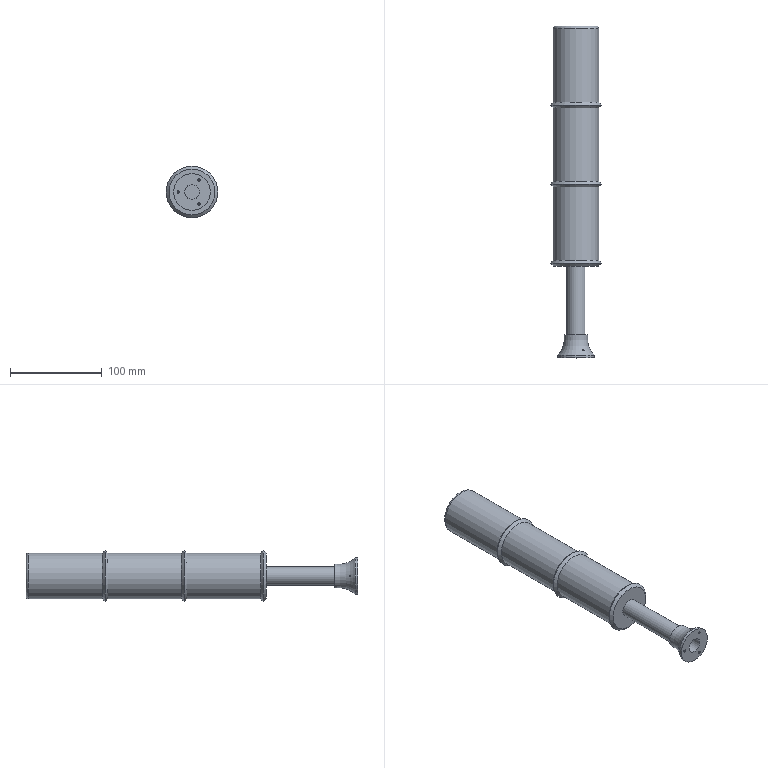Part | STEP file | Three-colour light | 1 solid | 25 faces | box 56 x 361 x 56 mm | volume 538523 mm3 | cylinder 9 | cone 9 | plane 5 | torus 2 | commonest cylinder face diameters 2.5 x3 50 x3 16 x1 20 x1 40 x1
STEP:
#1=CARTESIAN_POINT('',(0.,0.,-10.));
#2=VERTEX_POINT('',#1);
#3=CARTESIAN_POINT('',(0.,0.,0.));
#4=DIRECTION('',(0.,-1.,0.));
#5=DIRECTION('',(0.,0.,-1.));
#6=AXIS2_PLACEMENT_3D('',#3,#4,#5);
#7=CIRCLE('',#6,10.);
#8=EDGE_CURVE('',#2,#2,#7,.T.);
#9=ORIENTED_EDGE('',*,*,#8,.T.);
#10=EDGE_LOOP('',(#9));
#11=FACE_OUTER_BOUND('',#10,.T.);
#12=CARTESIAN_POINT('',(0.,-75.,-10.));
#13=VERTEX_POINT('',#12);
#14=CARTESIAN_POINT('',(0.,-75.,0.));
#15=DIRECTION('',(0.,-1.,0.));
#16=DIRECTION('',(0.,0.,-1.));
#17=AXIS2_PLACEMENT_3D('',#14,#15,#16);
#18=CIRCLE('',#17,10.);
#19=EDGE_CURVE('',#13,#13,#18,.T.);
#20=ORIENTED_EDGE('',*,*,#19,.F.);
#21=EDGE_LOOP('',(#20));
#22=FACE_OUTER_BOUND('',#21,.T.);
#23=CARTESIAN_POINT('',(0.,-100.,0.));
#24=DIRECTION('',(0.,1.,0.));
#25=DIRECTION('',(0.,0.,1.));
#26=AXIS2_PLACEMENT_3D('',#23,#24,#25);
#27=CYLINDRICAL_SURFACE('',#26,10.);
#28=ADVANCED_FACE('',(#11,#22),#27,.T.);
#29=CARTESIAN_POINT('',(0.,0.,-25.));
#30=VERTEX_POINT('',#29);
#31=CARTESIAN_POINT('',(0.,0.,0.));
#32=DIRECTION('',(0.,-1.,0.));
#33=DIRECTION('',(0.,0.,-1.));
#34=AXIS2_PLACEMENT_3D('',#31,#32,#33);
#35=CIRCLE('',#34,25.);
#36=EDGE_CURVE('',#30,#30,#35,.T.);
#37=ORIENTED_EDGE('',*,*,#36,.T.);
#38=EDGE_LOOP('',(#37));
#39=FACE_OUTER_BOUND('',#38,.T.);
#40=ORIENTED_EDGE('',*,*,#8,.F.);
#41=EDGE_LOOP('',(#40));
#42=FACE_BOUND('',#41,.T.);
#43=CARTESIAN_POINT('',(0.,0.,0.));
#44=DIRECTION('',(0.,-1.,0.));
#45=DIRECTION('',(0.,0.,-1.));
#46=AXIS2_PLACEMENT_3D('',#43,#44,#45);
#47=PLANE('',#46);
#48=ADVANCED_FACE('',(#39,#42),#47,.T.);
#49=CARTESIAN_POINT('',(0.,261.,-22.));
#50=VERTEX_POINT('',#49);
#51=CARTESIAN_POINT('',(0.,261.,0.));
#52=DIRECTION('',(0.,-1.,0.));
#53=DIRECTION('',(0.,0.,-1.));
#54=AXIS2_PLACEMENT_3D('',#51,#52,#53);
#55=CIRCLE('',#54,22.);
#56=EDGE_CURVE('',#50,#50,#55,.T.);
#57=ORIENTED_EDGE('',*,*,#56,.F.);
#58=EDGE_LOOP('',(#57));
#59=FACE_OUTER_BOUND('',#58,.T.);
#60=CARTESIAN_POINT('',(0.,261.,0.));
#61=DIRECTION('',(0.,1.,0.));
#62=DIRECTION('',(0.,0.,1.));
#63=AXIS2_PLACEMENT_3D('',#60,#61,#62);
#64=PLANE('',#63);
#65=ADVANCED_FACE('',(#59),#64,.T.);
#66=ORIENTED_EDGE('',*,*,#56,.T.);
#67=EDGE_LOOP('',(#66));
#68=FACE_OUTER_BOUND('',#67,.T.);
#69=CARTESIAN_POINT('',(0.,258.,-25.));
#70=VERTEX_POINT('',#69);
#71=CARTESIAN_POINT('',(0.,258.,0.));
#72=DIRECTION('',(0.,-1.,0.));
#73=DIRECTION('',(0.,0.,-1.));
#74=AXIS2_PLACEMENT_3D('',#71,#72,#73);
#75=CIRCLE('',#74,25.);
#76=EDGE_CURVE('',#70,#70,#75,.T.);
#77=ORIENTED_EDGE('',*,*,#76,.F.);
#78=EDGE_LOOP('',(#77));
#79=FACE_OUTER_BOUND('',#78,.T.);
#80=CARTESIAN_POINT('',(0.,258.,0.));
#81=DIRECTION('',(0.,-1.,0.));
#82=DIRECTION('',(0.,0.,-1.));
#83=AXIS2_PLACEMENT_3D('',#80,#81,#82);
#84=TOROIDAL_SURFACE('',#83,22.,3.);
#85=ADVANCED_FACE('',(#68,#79),#84,.T.);
#86=ORIENTED_EDGE('',*,*,#76,.T.);
#87=EDGE_LOOP('',(#86));
#88=FACE_OUTER_BOUND('',#87,.T.);
#89=CARTESIAN_POINT('',(0.,178.,-25.));
#90=VERTEX_POINT('',#89);
#91=CARTESIAN_POINT('',(0.,178.,0.));
#92=DIRECTION('',(0.,-1.,0.));
#93=DIRECTION('',(0.,0.,-1.));
#94=AXIS2_PLACEMENT_3D('',#91,#92,#93);
#95=CIRCLE('',#94,25.);
#96=EDGE_CURVE('',#90,#90,#95,.T.);
#97=ORIENTED_EDGE('',*,*,#96,.F.);
#98=EDGE_LOOP('',(#97));
#99=FACE_OUTER_BOUND('',#98,.T.);
#100=CARTESIAN_POINT('',(0.,0.,0.));
#101=DIRECTION('',(0.,-1.,0.));
#102=DIRECTION('',(0.,0.,-1.));
#103=AXIS2_PLACEMENT_3D('',#100,#101,#102);
#104=CYLINDRICAL_SURFACE('',#103,25.);
#105=ADVANCED_FACE('',(#88,#99),#104,.T.);
#106=ORIENTED_EDGE('',*,*,#96,.T.);
#107=EDGE_LOOP('',(#106));
#108=FACE_BOUND('',#107,.T.);
#109=CARTESIAN_POINT('',(0.,175.,-28.));
#110=VERTEX_POINT('',#109);
#111=CARTESIAN_POINT('',(0.,175.,0.));
#112=DIRECTION('',(0.,-1.,0.));
#113=DIRECTION('',(0.,0.,-1.));
#114=AXIS2_PLACEMENT_3D('',#111,#112,#113);
#115=CIRCLE('',#114,28.);
#116=EDGE_CURVE('',#110,#110,#115,.T.);
#117=ORIENTED_EDGE('',*,*,#116,.F.);
#118=EDGE_LOOP('',(#117));
#119=FACE_OUTER_BOUND('',#118,.T.);
#120=CARTESIAN_POINT('',(0.,175.,0.));
#121=DIRECTION('',(0.,-1.,0.));
#122=DIRECTION('',(0.,0.,-1.));
#123=AXIS2_PLACEMENT_3D('',#120,#121,#122);
#124=CONICAL_SURFACE('',#123,28.,0.7854);
#125=ADVANCED_FACE('',(#108,#119),#124,.T.);
#126=ORIENTED_EDGE('',*,*,#116,.T.);
#127=EDGE_LOOP('',(#126));
#128=FACE_OUTER_BOUND('',#127,.T.);
#129=CARTESIAN_POINT('',(0.,172.,-25.));
#130=VERTEX_POINT('',#129);
#131=CARTESIAN_POINT('',(0.,172.,0.));
#132=DIRECTION('',(0.,-1.,0.));
#133=DIRECTION('',(0.,0.,-1.));
#134=AXIS2_PLACEMENT_3D('',#131,#132,#133);
#135=CIRCLE('',#134,25.);
#136=EDGE_CURVE('',#130,#130,#135,.T.);
#137=ORIENTED_EDGE('',*,*,#136,.F.);
#138=EDGE_LOOP('',(#137));
#139=FACE_BOUND('',#138,.T.);
#140=CARTESIAN_POINT('',(0.,172.,0.));
#141=DIRECTION('',(0.,1.,0.));
#142=DIRECTION('',(0.,0.,1.));
#143=AXIS2_PLACEMENT_3D('',#140,#141,#142);
#144=CONICAL_SURFACE('',#143,25.,0.7854);
#145=ADVANCED_FACE('',(#128,#139),#144,.T.);
#146=ORIENTED_EDGE('',*,*,#136,.T.);
#147=EDGE_LOOP('',(#146));
#148=FACE_OUTER_BOUND('',#147,.T.);
#149=CARTESIAN_POINT('',(0.,92.,-25.));
#150=VERTEX_POINT('',#149);
#151=CARTESIAN_POINT('',(0.,92.,0.));
#152=DIRECTION('',(0.,-1.,0.));
#153=DIRECTION('',(0.,0.,-1.));
#154=AXIS2_PLACEMENT_3D('',#151,#152,#153);
#155=CIRCLE('',#154,25.);
#156=EDGE_CURVE('',#150,#150,#155,.T.);
#157=ORIENTED_EDGE('',*,*,#156,.F.);
#158=EDGE_LOOP('',(#157));
#159=FACE_OUTER_BOUND('',#158,.T.);
#160=CARTESIAN_POINT('',(0.,0.,0.));
#161=DIRECTION('',(0.,-1.,0.));
#162=DIRECTION('',(0.,0.,-1.));
#163=AXIS2_PLACEMENT_3D('',#160,#161,#162);
#164=CYLINDRICAL_SURFACE('',#163,25.);
#165=ADVANCED_FACE('',(#148,#159),#164,.T.);
#166=ORIENTED_EDGE('',*,*,#156,.T.);
#167=EDGE_LOOP('',(#166));
#168=FACE_BOUND('',#167,.T.);
#169=CARTESIAN_POINT('',(0.,89.,-28.));
#170=VERTEX_POINT('',#169);
#171=CARTESIAN_POINT('',(0.,89.,0.));
#172=DIRECTION('',(0.,-1.,0.));
#173=DIRECTION('',(0.,0.,-1.));
#174=AXIS2_PLACEMENT_3D('',#171,#172,#173);
#175=CIRCLE('',#174,28.);
#176=EDGE_CURVE('',#170,#170,#175,.T.);
#177=ORIENTED_EDGE('',*,*,#176,.F.);
#178=EDGE_LOOP('',(#177));
#179=FACE_OUTER_BOUND('',#178,.T.);
#180=CARTESIAN_POINT('',(0.,89.,0.));
#181=DIRECTION('',(0.,-1.,0.));
#182=DIRECTION('',(0.,0.,-1.));
#183=AXIS2_PLACEMENT_3D('',#180,#181,#182);
#184=CONICAL_SURFACE('',#183,28.,0.7854);
#185=ADVANCED_FACE('',(#168,#179),#184,.T.);
#186=ORIENTED_EDGE('',*,*,#176,.T.);
#187=EDGE_LOOP('',(#186));
#188=FACE_OUTER_BOUND('',#187,.T.);
#189=CARTESIAN_POINT('',(0.,86.,-25.));
#190=VERTEX_POINT('',#189);
#191=CARTESIAN_POINT('',(0.,86.,0.));
#192=DIRECTION('',(0.,-1.,0.));
#193=DIRECTION('',(0.,0.,-1.));
#194=AXIS2_PLACEMENT_3D('',#191,#192,#193);
#195=CIRCLE('',#194,25.);
#196=EDGE_CURVE('',#190,#190,#195,.T.);
#197=ORIENTED_EDGE('',*,*,#196,.F.);
#198=EDGE_LOOP('',(#197));
#199=FACE_BOUND('',#198,.T.);
#200=CARTESIAN_POINT('',(0.,86.,0.));
#201=DIRECTION('',(0.,1.,0.));
#202=DIRECTION('',(0.,0.,1.));
#203=AXIS2_PLACEMENT_3D('',#200,#201,#202);
#204=CONICAL_SURFACE('',#203,25.,0.7854);
#205=ADVANCED_FACE('',(#188,#199),#204,.T.);
#206=ORIENTED_EDGE('',*,*,#196,.T.);
#207=EDGE_LOOP('',(#206));
#208=FACE_OUTER_BOUND('',#207,.T.);
#209=CARTESIAN_POINT('',(0.,6.,-25.));
#210=VERTEX_POINT('',#209);
#211=CARTESIAN_POINT('',(0.,6.,0.));
#212=DIRECTION('',(0.,-1.,0.));
#213=DIRECTION('',(0.,0.,-1.));
#214=AXIS2_PLACEMENT_3D('',#211,#212,#213);
#215=CIRCLE('',#214,25.);
#216=EDGE_CURVE('',#210,#210,#215,.T.);
#217=ORIENTED_EDGE('',*,*,#216,.F.);
#218=EDGE_LOOP('',(#217));
#219=FACE_OUTER_BOUND('',#218,.T.);
#220=CARTESIAN_POINT('',(0.,0.,0.));
#221=DIRECTION('',(0.,-1.,0.));
#222=DIRECTION('',(0.,0.,-1.));
#223=AXIS2_PLACEMENT_3D('',#220,#221,#222);
#224=CYLINDRICAL_SURFACE('',#223,25.);
#225=ADVANCED_FACE('',(#208,#219),#224,.T.);
#226=ORIENTED_EDGE('',*,*,#216,.T.);
#227=EDGE_LOOP('',(#226));
#228=FACE_BOUND('',#227,.T.);
#229=CARTESIAN_POINT('',(0.,3.,-28.));
#230=VERTEX_POINT('',#229);
#231=CARTESIAN_POINT('',(0.,3.,0.));
#232=DIRECTION('',(0.,-1.,0.));
#233=DIRECTION('',(0.,0.,-1.));
#234=AXIS2_PLACEMENT_3D('',#231,#232,#233);
#235=CIRCLE('',#234,28.);
#236=EDGE_CURVE('',#230,#230,#235,.T.);
#237=ORIENTED_EDGE('',*,*,#236,.F.);
#238=EDGE_LOOP('',(#237));
#239=FACE_OUTER_BOUND('',#238,.T.);
#240=CARTESIAN_POINT('',(0.,3.,0.));
#241=DIRECTION('',(0.,-1.,0.));
#242=DIRECTION('',(0.,0.,-1.));
#243=AXIS2_PLACEMENT_3D('',#240,#241,#242);
#244=CONICAL_SURFACE('',#243,28.,0.7854);
#245=ADVANCED_FACE('',(#228,#239),#244,.T.);
#246=ORIENTED_EDGE('',*,*,#236,.T.);
#247=EDGE_LOOP('',(#246));
#248=FACE_OUTER_BOUND('',#247,.T.);
#249=ORIENTED_EDGE('',*,*,#36,.F.);
#250=EDGE_LOOP('',(#249));
#251=FACE_BOUND('',#250,.T.);
#252=CARTESIAN_POINT('',(0.,0.,0.));
#253=DIRECTION('',(0.,1.,0.));
#254=DIRECTION('',(0.,0.,1.));
#255=AXIS2_PLACEMENT_3D('',#252,#253,#254);
#256=CONICAL_SURFACE('',#255,25.,0.7854);
#257=ADVANCED_FACE('',(#248,#251),#256,.T.);
#258=CARTESIAN_POINT('',(0.,-97.,20.));
#259=VERTEX_POINT('',#258);
#260=CARTESIAN_POINT('',(0.,-97.,0.));
#261=DIRECTION('',(0.,1.,0.));
#262=DIRECTION('',(0.,0.,1.));
#263=AXIS2_PLACEMENT_3D('',#260,#261,#262);
#264=CIRCLE('',#263,20.);
#265=EDGE_CURVE('',#259,#259,#264,.T.);
#266=ORIENTED_EDGE('',*,*,#265,.F.);
#267=EDGE_LOOP('',(#266));
#268=FACE_OUTER_BOUND('',#267,.T.);
#269=CARTESIAN_POINT('',(0.,-100.,20.));
#270=VERTEX_POINT('',#269);
#271=CARTESIAN_POINT('',(0.,-100.,0.));
#272=DIRECTION('',(0.,1.,0.));
#273=DIRECTION('',(0.,0.,1.));
#274=AXIS2_PLACEMENT_3D('',#271,#272,#273);
#275=CIRCLE('',#274,20.);
#276=EDGE_CURVE('',#270,#270,#275,.T.);
#277=ORIENTED_EDGE('',*,*,#276,.T.);
#278=EDGE_LOOP('',(#277));
#279=FACE_OUTER_BOUND('',#278,.T.);
#280=CARTESIAN_POINT('',(0.,-100.,0.));
#281=DIRECTION('',(0.,1.,0.));
#282=DIRECTION('',(0.,0.,1.));
#283=AXIS2_PLACEMENT_3D('',#280,#281,#282);
#284=CYLINDRICAL_SURFACE('',#283,20.);
#285=ADVANCED_FACE('',(#268,#279),#284,.T.);
#286=CARTESIAN_POINT('',(8.733,-91.5,-13.196));
#287=VERTEX_POINT('',#286);
#288=CARTESIAN_POINT('',(7.061,-91.5,-14.161));
#289=VERTEX_POINT('',#288);
#290=CARTESIAN_POINT('',(8.733,-91.5,-13.196));
#291=CARTESIAN_POINT('',(8.583,-91.415,-13.238));
#292=CARTESIAN_POINT('',(8.432,-91.332,-13.28));
#293=CARTESIAN_POINT('',(8.2,-91.222,-13.354));
#294=CARTESIAN_POINT('',(8.122,-91.188,-13.379));
#295=CARTESIAN_POINT('',(7.964,-91.135,-13.441));
#296=CARTESIAN_POINT('',(7.883,-91.118,-13.478));
#297=CARTESIAN_POINT('',(7.73,-91.118,-13.566));
#298=CARTESIAN_POINT('',(7.658,-91.135,-13.618));
#299=CARTESIAN_POINT('',(7.526,-91.188,-13.724));
#300=CARTESIAN_POINT('',(7.464,-91.222,-13.778));
#301=CARTESIAN_POINT('',(7.285,-91.332,-13.942));
#302=CARTESIAN_POINT('',(7.173,-91.415,-14.052));
#303=CARTESIAN_POINT('',(7.061,-91.5,-14.161));
#304=B_SPLINE_CURVE_WITH_KNOTS('',3,(#290,#291,#292,#293,#294,#295,#296,#297,#298,#299,#300,#301,#302,#303),.UNSPECIFIED.,.F.,.F.,(4,2,2,2,2,2,4),(0.000000419,0.0005336,0.0008002,0.001067,0.001333,0.0016,0.002133),.UNSPECIFIED.);
#305=EDGE_CURVE('',#287,#289,#304,.T.);
#306=ORIENTED_EDGE('',*,*,#305,.T.);
#307=CARTESIAN_POINT('',(7.061,-91.5,-14.161));
#308=CARTESIAN_POINT('',(7.126,-91.591,-14.185));
#309=CARTESIAN_POINT('',(7.196,-91.678,-14.205));
#310=CARTESIAN_POINT('',(7.349,-91.842,-14.234));
#311=CARTESIAN_POINT('',(7.433,-91.92,-14.242));
#312=CARTESIAN_POINT('',(7.615,-92.059,-14.238));
#313=CARTESIAN_POINT('',(7.714,-92.12,-14.226));
#314=CARTESIAN_POINT('',(7.918,-92.206,-14.173));
#315=CARTESIAN_POINT('',(8.025,-92.231,-14.13));
#316=CARTESIAN_POINT('',(8.222,-92.231,-14.017));
#317=CARTESIAN_POINT('',(8.313,-92.207,-13.946));
#318=CARTESIAN_POINT('',(8.463,-92.121,-13.795));
#319=CARTESIAN_POINT('',(8.522,-92.061,-13.716));
#320=CARTESIAN_POINT('',(8.664,-91.853,-13.481));
#321=CARTESIAN_POINT('',(8.71,-91.682,-13.333));
#322=CARTESIAN_POINT('',(8.733,-91.5,-13.196));
#323=B_SPLINE_CURVE_WITH_KNOTS('',3,(#307,#308,#309,#310,#311,#312,#313,#314,#315,#316,#317,#318,#319,#320,#321,#322),.UNSPECIFIED.,.F.,.F.,(4,2,2,2,2,2,2,4),(0.000000249,0.0003396,0.0006789,0.001018,0.001358,0.001697,0.002036,0.002715),.UNSPECIFIED.);
#324=EDGE_CURVE('',#289,#287,#323,.T.);
#325=ORIENTED_EDGE('',*,*,#324,.T.);
#326=EDGE_LOOP('',(#306,#325));
#327=FACE_BOUND('',#326,.T.);
#328=CARTESIAN_POINT('',(7.061,-91.5,14.161));
#329=VERTEX_POINT('',#328);
#330=CARTESIAN_POINT('',(8.733,-91.5,13.196));
#331=VERTEX_POINT('',#330);
#332=CARTESIAN_POINT('',(7.061,-91.5,14.161));
#333=CARTESIAN_POINT('',(7.173,-91.415,14.052));
#334=CARTESIAN_POINT('',(7.285,-91.332,13.942));
#335=CARTESIAN_POINT('',(7.465,-91.222,13.778));
#336=CARTESIAN_POINT('',(7.526,-91.188,13.724));
#337=CARTESIAN_POINT('',(7.658,-91.135,13.618));
#338=CARTESIAN_POINT('',(7.731,-91.118,13.566));
#339=CARTESIAN_POINT('',(7.884,-91.118,13.478));
#340=CARTESIAN_POINT('',(7.965,-91.135,13.441));
#341=CARTESIAN_POINT('',(8.122,-91.188,13.379));
#342=CARTESIAN_POINT('',(8.2,-91.222,13.353));
#343=CARTESIAN_POINT('',(8.432,-91.332,13.28));
#344=CARTESIAN_POINT('',(8.583,-91.415,13.238));
#345=CARTESIAN_POINT('',(8.733,-91.5,13.196));
#346=B_SPLINE_CURVE_WITH_KNOTS('',3,(#332,#333,#334,#335,#336,#337,#338,#339,#340,#341,#342,#343,#344,#345),.UNSPECIFIED.,.F.,.F.,(4,2,2,2,2,2,4),(0.000000419,0.0005336,0.0008002,0.001067,0.001333,0.0016,0.002133),.UNSPECIFIED.);
#347=EDGE_CURVE('',#329,#331,#346,.T.);
#348=ORIENTED_EDGE('',*,*,#347,.T.);
#349=CARTESIAN_POINT('',(8.733,-91.5,13.196));
#350=CARTESIAN_POINT('',(8.722,-91.591,13.264));
#351=CARTESIAN_POINT('',(8.704,-91.678,13.335));
#352=CARTESIAN_POINT('',(8.652,-91.842,13.481));
#353=CARTESIAN_POINT('',(8.618,-91.92,13.558));
#354=CARTESIAN_POINT('',(8.523,-92.059,13.714));
#355=CARTESIAN_POINT('',(8.464,-92.12,13.794));
#356=CARTESIAN_POINT('',(8.315,-92.206,13.944));
#357=CARTESIAN_POINT('',(8.225,-92.231,14.015));
#358=CARTESIAN_POINT('',(8.028,-92.231,14.129));
#359=CARTESIAN_POINT('',(7.921,-92.207,14.172));
#360=CARTESIAN_POINT('',(7.715,-92.121,14.226));
#361=CARTESIAN_POINT('',(7.617,-92.061,14.238));
#362=CARTESIAN_POINT('',(7.343,-91.853,14.244));
#363=CARTESIAN_POINT('',(7.192,-91.682,14.21));
#364=CARTESIAN_POINT('',(7.061,-91.5,14.161));
#365=B_SPLINE_CURVE_WITH_KNOTS('',3,(#349,#350,#351,#352,#353,#354,#355,#356,#357,#358,#359,#360,#361,#362,#363,#364),.UNSPECIFIED.,.F.,.F.,(4,2,2,2,2,2,2,4),(0.000000249,0.0003396,0.0006789,0.001018,0.001358,0.001697,0.002036,0.002715),.UNSPECIFIED.);
#366=EDGE_CURVE('',#331,#329,#365,.T.);
#367=ORIENTED_EDGE('',*,*,#366,.T.);
#368=EDGE_LOOP('',(#348,#367));
#369=FACE_BOUND('',#368,.T.);
#370=CARTESIAN_POINT('',(-15.794,-91.5,0.9652));
#371=VERTEX_POINT('',#370);
#372=CARTESIAN_POINT('',(-15.794,-91.5,-0.9652));
#373=VERTEX_POINT('',#372);
#374=CARTESIAN_POINT('',(-15.794,-91.5,0.9652));
#375=CARTESIAN_POINT('',(-15.848,-91.591,0.921));
#376=CARTESIAN_POINT('',(-15.9,-91.678,0.8705));
#377=CARTESIAN_POINT('',(-16.001,-91.842,0.7523));
#378=CARTESIAN_POINT('',(-16.05,-91.92,0.6841));
#379=CARTESIAN_POINT('',(-16.138,-92.059,0.5244));
#380=CARTESIAN_POINT('',(-16.177,-92.12,0.4328));
#381=CARTESIAN_POINT('',(-16.233,-92.206,0.2294));
#382=CARTESIAN_POINT('',(-16.25,-92.231,0.1154));
#383=CARTESIAN_POINT('',(-16.25,-92.231,-0.1119));
#384=CARTESIAN_POINT('',(-16.234,-92.207,-0.2263));
#385=CARTESIAN_POINT('',(-16.178,-92.121,-0.4318));
#386=CARTESIAN_POINT('',(-16.139,-92.061,-0.5225));
#387=CARTESIAN_POINT('',(-16.007,-91.853,-0.7624));
#388=CARTESIAN_POINT('',(-15.902,-91.682,-0.8767));
#389=CARTESIAN_POINT('',(-15.794,-91.5,-0.9652));
#390=B_SPLINE_CURVE_WITH_KNOTS('',3,(#374,#375,#376,#377,#378,#379,#380,#381,#382,#383,#384,#385,#386,#387,#388,#389),.UNSPECIFIED.,.F.,.F.,(4,2,2,2,2,2,2,4),(0.000000249,0.0003396,0.0006789,0.001018,0.001358,0.001697,0.002036,0.002715),.UNSPECIFIED.);
#391=EDGE_CURVE('',#371,#373,#390,.T.);
#392=ORIENTED_EDGE('',*,*,#391,.T.);
#393=CARTESIAN_POINT('',(-15.794,-91.5,-0.9652));
#394=CARTESIAN_POINT('',(-15.756,-91.415,-0.8138));
#395=CARTESIAN_POINT('',(-15.717,-91.332,-0.6617));
#396=CARTESIAN_POINT('',(-15.664,-91.222,-0.4244));
#397=CARTESIAN_POINT('',(-15.648,-91.188,-0.3441));
#398=CARTESIAN_POINT('',(-15.622,-91.135,-0.1766));
#399=CARTESIAN_POINT('',(-15.614,-91.118,-0.08814));
#400=CARTESIAN_POINT('',(-15.614,-91.118,0.08857));
#401=CARTESIAN_POINT('',(-15.623,-91.135,0.1773));
#402=CARTESIAN_POINT('',(-15.648,-91.188,0.3443));
#403=CARTESIAN_POINT('',(-15.665,-91.222,0.4252));
#404=CARTESIAN_POINT('',(-15.717,-91.332,0.6621));
#405=CARTESIAN_POINT('',(-15.756,-91.415,0.814));
#406=CARTESIAN_POINT('',(-15.794,-91.5,0.9652));
#407=B_SPLINE_CURVE_WITH_KNOTS('',3,(#393,#394,#395,#396,#397,#398,#399,#400,#401,#402,#403,#404,#405,#406),.UNSPECIFIED.,.F.,.F.,(4,2,2,2,2,2,4),(0.000000419,0.0005336,0.0008002,0.001067,0.001333,0.0016,0.002133),.UNSPECIFIED.);
#408=EDGE_CURVE('',#373,#371,#407,.T.);
#409=ORIENTED_EDGE('',*,*,#408,.T.);
#410=EDGE_LOOP('',(#392,#409));
#411=FACE_BOUND('',#410,.T.);
#412=CARTESIAN_POINT('',(0.,-75.,13.));
#413=VERTEX_POINT('',#412);
#414=CARTESIAN_POINT('',(0.,-75.,0.));
#415=DIRECTION('',(0.,1.,0.));
#416=DIRECTION('',(0.,0.,1.));
#417=AXIS2_PLACEMENT_3D('',#414,#415,#416);
#418=CIRCLE('',#417,13.);
#419=EDGE_CURVE('',#413,#413,#418,.T.);
#420=ORIENTED_EDGE('',*,*,#419,.F.);
#421=EDGE_LOOP('',(#420));
#422=FACE_OUTER_BOUND('',#421,.T.);
#423=ORIENTED_EDGE('',*,*,#265,.T.);
#424=EDGE_LOOP('',(#423));
#425=FACE_OUTER_BOUND('',#424,.T.);
#426=CARTESIAN_POINT('',(0.,-79.276,0.));
#427=DIRECTION('',(0.,1.,0.));
#428=DIRECTION('',(0.,0.,1.));
#429=AXIS2_PLACEMENT_3D('',#426,#427,#428);
#430=TOROIDAL_SURFACE('',#429,37.632,25.);
#431=ADVANCED_FACE('',(#327,#369,#411,#422,#425),#430,.F.);
#432=ORIENTED_EDGE('',*,*,#19,.T.);
#433=EDGE_LOOP('',(#432));
#434=FACE_BOUND('',#433,.T.);
#435=ORIENTED_EDGE('',*,*,#419,.T.);
#436=EDGE_LOOP('',(#435));
#437=FACE_OUTER_BOUND('',#436,.T.);
#438=CARTESIAN_POINT('',(0.,-75.,-10.));
#439=DIRECTION('',(0.,-1.,0.));
#440=DIRECTION('',(0.,0.,-1.));
#441=AXIS2_PLACEMENT_3D('',#438,#439,#440);
#442=PLANE('',#441);
#443=ADVANCED_FACE('',(#434,#437),#442,.F.);
#444=CARTESIAN_POINT('',(0.,0.,-8.));
#445=VERTEX_POINT('',#444);
#446=CARTESIAN_POINT('',(0.,0.,0.));
#447=DIRECTION('',(0.,1.,0.));
#448=DIRECTION('',(0.,0.,-1.));
#449=AXIS2_PLACEMENT_3D('',#446,#447,#448);
#450=CIRCLE('',#449,8.);
#451=EDGE_CURVE('',#445,#445,#450,.T.);
#452=ORIENTED_EDGE('',*,*,#451,.F.);
#453=EDGE_LOOP('',(#452));
#454=FACE_OUTER_BOUND('',#453,.T.);
#455=CARTESIAN_POINT('',(0.,0.,0.));
#456=DIRECTION('',(0.,-1.,0.));
#457=DIRECTION('',(0.,0.,-1.));
#458=AXIS2_PLACEMENT_3D('',#455,#456,#457);
#459=PLANE('',#458);
#460=ADVANCED_FACE('',(#454),#459,.T.);
#461=CARTESIAN_POINT('',(8.,-100.,0.));
#462=VERTEX_POINT('',#461);
#463=CARTESIAN_POINT('',(0.,-100.,0.));
#464=DIRECTION('',(0.,-1.,0.));
#465=DIRECTION('',(1.,0.,0.));
#466=AXIS2_PLACEMENT_3D('',#463,#464,#465);
#467=CIRCLE('',#466,8.);
#468=EDGE_CURVE('',#462,#462,#467,.T.);
#469=ORIENTED_EDGE('',*,*,#468,.T.);
#470=EDGE_LOOP('',(#469));
#471=FACE_OUTER_BOUND('',#470,.T.);
#472=ORIENTED_EDGE('',*,*,#451,.T.);
#473=EDGE_LOOP('',(#472));
#474=FACE_OUTER_BOUND('',#473,.T.);
#475=CARTESIAN_POINT('',(0.,-100.,0.));
#476=DIRECTION('',(0.,1.,0.));
#477=DIRECTION('',(0.,0.,1.));
#478=AXIS2_PLACEMENT_3D('',#475,#476,#477);
#479=CYLINDRICAL_SURFACE('',#478,8.);
#480=ADVANCED_FACE('',(#471,#474),#479,.F.);
#481=CARTESIAN_POINT('',(7.5,-100.,-14.24));
#482=VERTEX_POINT('',#481);
#483=CARTESIAN_POINT('',(7.5,-100.,-12.99));
#484=DIRECTION('',(0.,-1.,0.));
#485=DIRECTION('',(0.,0.,-1.));
#486=AXIS2_PLACEMENT_3D('',#483,#484,#485);
#487=CIRCLE('',#486,1.25);
#488=EDGE_CURVE('',#482,#482,#487,.T.);
#489=ORIENTED_EDGE('',*,*,#488,.F.);
#490=EDGE_LOOP('',(#489));
#491=FACE_BOUND('',#490,.T.);
#492=CARTESIAN_POINT('',(7.5,-100.,11.74));
#493=VERTEX_POINT('',#492);
#494=CARTESIAN_POINT('',(7.5,-100.,12.99));
#495=DIRECTION('',(0.,-1.,0.));
#496=DIRECTION('',(0.,0.,-1.));
#497=AXIS2_PLACEMENT_3D('',#494,#495,#496);
#498=CIRCLE('',#497,1.25);
#499=EDGE_CURVE('',#493,#493,#498,.T.);
#500=ORIENTED_EDGE('',*,*,#499,.F.);
#501=EDGE_LOOP('',(#500));
#502=FACE_BOUND('',#501,.T.);
#503=CARTESIAN_POINT('',(-15.,-100.,-1.25));
#504=VERTEX_POINT('',#503);
#505=CARTESIAN_POINT('',(-15.,-100.,0.));
#506=DIRECTION('',(0.,-1.,0.));
#507=DIRECTION('',(0.,0.,-1.));
#508=AXIS2_PLACEMENT_3D('',#505,#506,#507);
#509=CIRCLE('',#508,1.25);
#510=EDGE_CURVE('',#504,#504,#509,.T.);
#511=ORIENTED_EDGE('',*,*,#510,.F.);
#512=EDGE_LOOP('',(#511));
#513=FACE_BOUND('',#512,.T.);
#514=ORIENTED_EDGE('',*,*,#468,.F.);
#515=EDGE_LOOP('',(#514));
#516=FACE_BOUND('',#515,.T.);
#517=ORIENTED_EDGE('',*,*,#276,.F.);
#518=EDGE_LOOP('',(#517));
#519=FACE_OUTER_BOUND('',#518,.T.);
#520=CARTESIAN_POINT('',(0.,-100.,0.));
#521=DIRECTION('',(0.,-1.,0.));
#522=DIRECTION('',(0.,0.,-1.));
#523=AXIS2_PLACEMENT_3D('',#520,#521,#522);
#524=PLANE('',#523);
#525=ADVANCED_FACE('',(#491,#502,#513,#516,#519),#524,.T.);
#526=CARTESIAN_POINT('',(-15.,-91.5,0.));
#527=DIRECTION('',(0.,-1.,0.));
#528=DIRECTION('',(0.,0.,-1.));
#529=AXIS2_PLACEMENT_3D('',#526,#527,#528);
#530=CIRCLE('',#529,1.25);
#531=EDGE_CURVE('',#373,#371,#530,.T.);
#532=ORIENTED_EDGE('',*,*,#531,.T.);
#533=ORIENTED_EDGE('',*,*,#408,.F.);
#534=EDGE_LOOP('',(#532,#533));
#535=FACE_OUTER_BOUND('',#534,.T.);
#536=CARTESIAN_POINT('',(-15.,-91.5,0.));
#537=DIRECTION('',(0.,-1.,0.));
#538=DIRECTION('',(0.,0.,-1.));
#539=AXIS2_PLACEMENT_3D('',#536,#537,#538);
#540=CONICAL_SURFACE('',#539,1.25,1.03);
#541=ADVANCED_FACE('',(#535),#540,.F.);
#542=ORIENTED_EDGE('',*,*,#510,.T.);
#543=EDGE_LOOP('',(#542));
#544=FACE_OUTER_BOUND('',#543,.T.);
#545=ORIENTED_EDGE('',*,*,#531,.F.);
#546=ORIENTED_EDGE('',*,*,#391,.F.);
#547=EDGE_LOOP('',(#545,#546));
#548=FACE_OUTER_BOUND('',#547,.T.);
#549=CARTESIAN_POINT('',(-15.,-100.,0.));
#550=DIRECTION('',(0.,-1.,0.));
#551=DIRECTION('',(0.,0.,-1.));
#552=AXIS2_PLACEMENT_3D('',#549,#550,#551);
#553=CYLINDRICAL_SURFACE('',#552,1.25);
#554=ADVANCED_FACE('',(#544,#548),#553,.F.);
#555=ORIENTED_EDGE('',*,*,#499,.T.);
#556=EDGE_LOOP('',(#555));
#557=FACE_OUTER_BOUND('',#556,.T.);
#558=CARTESIAN_POINT('',(7.5,-91.5,12.99));
#559=DIRECTION('',(0.,-1.,0.));
#560=DIRECTION('',(0.,0.,-1.));
#561=AXIS2_PLACEMENT_3D('',#558,#559,#560);
#562=CIRCLE('',#561,1.25);
#563=EDGE_CURVE('',#329,#331,#562,.T.);
#564=ORIENTED_EDGE('',*,*,#563,.F.);
#565=ORIENTED_EDGE('',*,*,#366,.F.);
#566=EDGE_LOOP('',(#564,#565));
#567=FACE_OUTER_BOUND('',#566,.T.);
#568=CARTESIAN_POINT('',(7.5,-100.,12.99));
#569=DIRECTION('',(0.,-1.,0.));
#570=DIRECTION('',(0.,0.,-1.));
#571=AXIS2_PLACEMENT_3D('',#568,#569,#570);
#572=CYLINDRICAL_SURFACE('',#571,1.25);
#573=ADVANCED_FACE('',(#557,#567),#572,.F.);
#574=ORIENTED_EDGE('',*,*,#563,.T.);
#575=ORIENTED_EDGE('',*,*,#347,.F.);
#576=EDGE_LOOP('',(#574,#575));
#577=FACE_OUTER_BOUND('',#576,.T.);
#578=CARTESIAN_POINT('',(7.5,-91.5,12.99));
#579=DIRECTION('',(0.,-1.,0.));
#580=DIRECTION('',(0.,0.,-1.));
#581=AXIS2_PLACEMENT_3D('',#578,#579,#580);
#582=CONICAL_SURFACE('',#581,1.25,1.03);
#583=ADVANCED_FACE('',(#577),#582,.F.);
#584=ORIENTED_EDGE('',*,*,#488,.T.);
#585=EDGE_LOOP('',(#584));
#586=FACE_OUTER_BOUND('',#585,.T.);
#587=CARTESIAN_POINT('',(7.5,-91.5,-12.99));
#588=DIRECTION('',(0.,-1.,0.));
#589=DIRECTION('',(0.,0.,-1.));
#590=AXIS2_PLACEMENT_3D('',#587,#588,#589);
#591=CIRCLE('',#590,1.25);
#592=EDGE_CURVE('',#287,#289,#591,.T.);
#593=ORIENTED_EDGE('',*,*,#592,.F.);
#594=ORIENTED_EDGE('',*,*,#324,.F.);
#595=EDGE_LOOP('',(#593,#594));
#596=FACE_OUTER_BOUND('',#595,.T.);
#597=CARTESIAN_POINT('',(7.5,-100.,-12.99));
#598=DIRECTION('',(0.,-1.,0.));
#599=DIRECTION('',(0.,0.,-1.));
#600=AXIS2_PLACEMENT_3D('',#597,#598,#599);
#601=CYLINDRICAL_SURFACE('',#600,1.25);
#602=ADVANCED_FACE('',(#586,#596),#601,.F.);
#603=ORIENTED_EDGE('',*,*,#592,.T.);
#604=ORIENTED_EDGE('',*,*,#305,.F.);
#605=EDGE_LOOP('',(#603,#604));
#606=FACE_OUTER_BOUND('',#605,.T.);
#607=CARTESIAN_POINT('',(7.5,-91.5,-12.99));
#608=DIRECTION('',(0.,-1.,0.));
#609=DIRECTION('',(0.,0.,-1.));
#610=AXIS2_PLACEMENT_3D('',#607,#608,#609);
#611=CONICAL_SURFACE('',#610,1.25,1.03);
#612=ADVANCED_FACE('',(#606),#611,.F.);
#613=CLOSED_SHELL('',(#28,#48,#65,#85,#105,#125,#145,#165,#185,#205,#225,#245,#257,#285,#431,#443,#460,#480,#525,#541,#554,#573,#583,#602,#612));
#614=MANIFOLD_SOLID_BREP('',#613);
#615=CARTESIAN_POINT('',(0.,0.,0.));
#616=DIRECTION('',(0.,0.,1.));
#617=DIRECTION('',(1.,0.,0.));
#618=AXIS2_PLACEMENT_3D('',#615,#616,#617);
#619=(LENGTH_UNIT()NAMED_UNIT(*)SI_UNIT(.MILLI.,.METRE.));
#620=UNCERTAINTY_MEASURE_WITH_UNIT(LENGTH_MEASURE(0.00001),#619,'','');
#621=(NAMED_UNIT(*)PLANE_ANGLE_UNIT()SI_UNIT($,.RADIAN.));
#622=(NAMED_UNIT(*)SI_UNIT($,.STERADIAN.)SOLID_ANGLE_UNIT());
#623=(GEOMETRIC_REPRESENTATION_CONTEXT(3)GLOBAL_UNCERTAINTY_ASSIGNED_CONTEXT((#620))GLOBAL_UNIT_ASSIGNED_CONTEXT((#619,#621,#622))REPRESENTATION_CONTEXT('',''));
#624=ADVANCED_BREP_SHAPE_REPRESENTATION('',(#614,#618),#623);